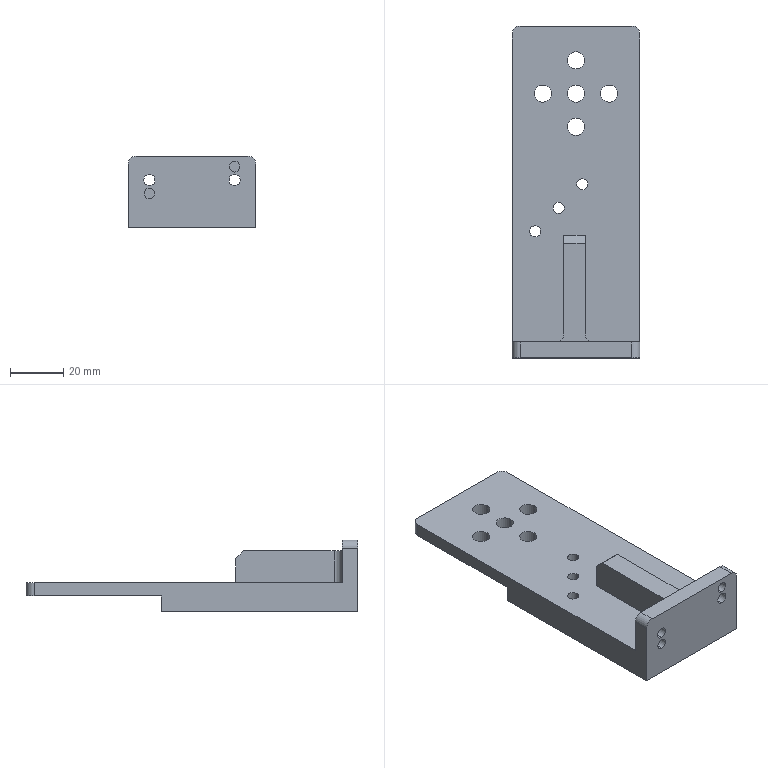NC program | NX | posted with a generic post | part box 48 x 124.7 x 27 mm
Lines 1859 to 3165 of 3165:
(ZLEVEL_PROFILE , TOOL : D6)
N3698 T12 M6
N3700 G54
N3702 G17 G0 G90 X-52.15 Y10.619 B0. C0. S9500 M3
N3704 G43 Z30. H12
N3706 Z-4.5
N3708 G94 G1 X-53.05 Y10.099 F1600.
N3710 G3 X-53.35 Y9.58 R0.6
N3712 G1 Y7.573
N3714 X-51.344
N3716 G3 X-50.824 Y7.873 R0.6
N3718 G1 X-50.304 Y8.773
N3720 G0 X-52.15 Y10.619 Z-5.
N3722 G1 X-53.05 Y10.099
N3724 G3 X-53.35 Y9.58 R0.6
N3726 G1 Y7.573
N3728 X-51.344
N3730 G3 X-50.824 Y7.873 R0.6
N3732 G1 X-50.304 Y8.773
N3734 G0 X-52.15 Y10.619 Z-5.5
N3736 G1 X-53.05 Y10.099
N3738 G3 X-53.35 Y9.58 R0.6
N3740 G1 Y7.573
N3742 X-51.344
N3744 G3 X-50.824 Y7.873 R0.6
N3746 G1 X-50.304 Y8.773
N3748 G0 X-52.15 Y10.619 Z-6.
N3750 G1 X-53.05 Y10.099
N3752 G3 X-53.35 Y9.58 R0.6
N3754 G1 Y7.573
N3756 X-51.344
N3758 G3 X-50.824 Y7.873 R0.6
N3760 G1 X-50.304 Y8.773
N3762 G0 X-52.15 Y10.619 Z-6.5
N3764 G1 X-53.05 Y10.099
N3766 G3 X-53.35 Y9.58 R0.6
N3768 G1 Y7.573
N3770 X-51.344
N3772 G3 X-50.824 Y7.873 R0.6
N3774 G1 X-50.304 Y8.773
N3776 G0 X-52.15 Y10.619 Z-7.
N3778 G1 X-53.05 Y10.099
N3780 G3 X-53.35 Y9.58 R0.6
N3782 G1 Y7.573
N3784 X-51.344
N3786 G3 X-50.824 Y7.873 R0.6
N3788 G1 X-50.304 Y8.773
N3790 G0 X-52.15 Y10.619 Z-7.5
N3792 G1 X-53.05 Y10.099
N3794 G3 X-53.35 Y9.58 R0.6
N3796 G1 Y7.573
N3798 X-51.344
N3800 G3 X-50.824 Y7.873 R0.6
N3802 G1 X-50.304 Y8.773
N3804 G0 X-52.15 Y10.619 Z-8.
N3806 G1 X-53.05 Y10.099
N3808 G3 X-53.35 Y9.58 R0.6
N3810 G1 Y7.573
N3812 X-51.344
N3814 G3 X-50.824 Y7.873 R0.6
N3816 G1 X-50.304 Y8.773
N3818 G0 X-52.15 Y10.619 Z-8.5
N3820 G1 X-53.05 Y10.099
N3822 G3 X-53.35 Y9.58 R0.6
N3824 G1 Y7.573
N3826 X-51.344
N3828 G3 X-50.824 Y7.873 R0.6
N3830 G1 X-50.304 Y8.773
N3832 G0 X-52.15 Y10.619 Z-9.
N3834 G1 X-53.05 Y10.099
N3836 G3 X-53.35 Y9.58 R0.6
N3838 G1 Y7.573
N3840 X-51.344
N3842 G3 X-50.824 Y7.873 R0.6
N3844 G1 X-50.304 Y8.773
N3846 G0 X-52.15 Y10.619 Z-9.5
N3848 G1 X-53.05 Y10.099
N3850 G3 X-53.35 Y9.58 R0.6
N3852 G1 Y7.573
N3854 X-51.344
N3856 G3 X-50.824 Y7.873 R0.6
N3858 G1 X-50.304 Y8.773
N3860 G0 X-52.15 Y10.619 Z-10.
N3862 G1 X-53.05 Y10.099
N3864 G3 X-53.35 Y9.58 R0.6
N3866 G1 Y7.573
N3868 X-51.344
N3870 G3 X-50.824 Y7.873 R0.6
N3872 G1 X-50.304 Y8.773
N3874 G0 X-52.15 Y10.619 Z-10.5
N3876 G1 X-53.05 Y10.099
N3878 G3 X-53.35 Y9.58 R0.6
N3880 G1 Y7.573
N3882 X-51.344
N3884 G3 X-50.824 Y7.873 R0.6
N3886 G1 X-50.304 Y8.773
N3888 G0 X-52.15 Y10.619 Z-11.
N3890 G1 X-53.05 Y10.099
N3892 G3 X-53.35 Y9.58 R0.6
N3894 G1 Y7.573
N3896 X-51.344
N3898 G3 X-50.824 Y7.873 R0.6
N3900 G1 X-50.304 Y8.773
N3902 G0 X-52.15 Y10.619 Z-11.5
N3904 G1 X-53.05 Y10.099
N3906 G3 X-53.35 Y9.58 R0.6
N3908 G1 Y7.573
N3910 X-51.344
N3912 G3 X-50.824 Y7.873 R0.6
N3914 G1 X-50.304 Y8.773
N3916 G0 X-52.15 Y10.619 Z-12.
N3918 G1 X-53.05 Y10.099
N3920 G3 X-53.35 Y9.58 R0.6
N3922 G1 Y7.573
N3924 X-51.344
N3926 G3 X-50.824 Y7.873 R0.6
N3928 G1 X-50.304 Y8.773
N3930 G0 X-52.15 Y10.619 Z-12.5
N3932 G1 X-53.05 Y10.099
N3934 G3 X-53.35 Y9.58 R0.6
N3936 G1 Y7.573
N3938 X-51.344
N3940 G3 X-50.824 Y7.873 R0.6
N3942 G1 X-50.304 Y8.773
N3944 G0 X-52.15 Y10.619 Z-13.
N3946 G1 X-53.05 Y10.099
N3948 G3 X-53.35 Y9.58 R0.6
N3950 G1 Y7.573
N3952 X-51.344
N3954 G3 X-50.824 Y7.873 R0.6
N3956 G1 X-50.304 Y8.773
N3958 G0 X-52.15 Y10.619 Z-13.5
N3960 G1 X-53.05 Y10.099
N3962 G3 X-53.35 Y9.58 R0.6
N3964 G1 Y7.573
N3966 X-51.344
N3968 G3 X-50.824 Y7.873 R0.6
N3970 G1 X-50.304 Y8.773
N3972 G0 X-52.15 Y10.619 Z-14.
N3974 G1 X-53.05 Y10.099
N3976 G3 X-53.35 Y9.58 R0.6
N3978 G1 Y7.573
N3980 X-51.344
N3982 G3 X-50.824 Y7.873 R0.6
N3984 G1 X-50.304 Y8.773
N3986 G0 X-52.15 Y10.619 Z-14.5
N3988 G1 X-53.05 Y10.099
N3990 G3 X-53.35 Y9.58 R0.6
N3992 G1 Y7.573
N3994 X-51.344
N3996 G3 X-50.824 Y7.873 R0.6
N3998 G1 X-50.304 Y8.773
N4000 G0 X-52.15 Y10.619 Z-15.
N4002 G1 X-53.05 Y10.099
N4004 G3 X-53.35 Y9.58 R0.6
N4006 G1 Y7.573
N4008 X-51.344
N4010 G3 X-50.824 Y7.873 R0.6
N4012 G1 X-50.304 Y8.773
N4014 G0 X-52.15 Y10.619 Z-15.5
N4016 G1 X-53.05 Y10.099
N4018 G3 X-53.35 Y9.58 R0.6
N4020 G1 Y7.573
N4022 X-51.344
N4024 G3 X-50.824 Y7.873 R0.6
N4026 G1 X-50.304 Y8.773
N4028 G0 X-52.15 Y10.619 Z-16.
N4030 G1 X-53.05 Y10.099
N4032 G3 X-53.35 Y9.58 R0.6
N4034 G1 Y7.573
N4036 X-51.344
N4038 G3 X-50.824 Y7.873 R0.6
N4040 G1 X-50.304 Y8.773
N4042 G0 Z30.
N4044 Y-7.627
N4046 Z-4.5
N4048 G1 X-50.824 Y-6.727
N4050 G3 X-51.344 Y-6.427 R0.6
N4052 G1 X-53.35
N4054 Y-8.433
N4056 G3 X-53.05 Y-8.953 R0.6
N4058 G1 X-52.15 Y-9.472
N4060 G0 X-50.304 Y-7.627 Z-5.
N4062 G1 X-50.824 Y-6.727
N4064 G3 X-51.344 Y-6.427 R0.6
N4066 G1 X-53.35
N4068 Y-8.433
N4070 G3 X-53.05 Y-8.953 R0.6
N4072 G1 X-52.15 Y-9.472
N4074 G0 X-50.304 Y-7.627 Z-5.5
N4076 G1 X-50.824 Y-6.727
N4078 G3 X-51.344 Y-6.427 R0.6
N4080 G1 X-53.35
N4082 Y-8.433
N4084 G3 X-53.05 Y-8.953 R0.6
N4086 G1 X-52.15 Y-9.472
N4088 G0 X-50.304 Y-7.627 Z-6.
N4090 G1 X-50.824 Y-6.727
N4092 G3 X-51.344 Y-6.427 R0.6
N4094 G1 X-53.35
N4096 Y-8.433
N4098 G3 X-53.05 Y-8.953 R0.6
N4100 G1 X-52.15 Y-9.472
N4102 G0 X-50.304 Y-7.627 Z-6.5
N4104 G1 X-50.824 Y-6.727
N4106 G3 X-51.344 Y-6.427 R0.6
N4108 G1 X-53.35
N4110 Y-8.433
N4112 G3 X-53.05 Y-8.953 R0.6
N4114 G1 X-52.15 Y-9.472
N4116 G0 X-50.304 Y-7.627 Z-7.
N4118 G1 X-50.824 Y-6.727
N4120 G3 X-51.344 Y-6.427 R0.6
N4122 G1 X-53.35
N4124 Y-8.433
N4126 G3 X-53.05 Y-8.953 R0.6
N4128 G1 X-52.15 Y-9.472
N4130 G0 X-50.304 Y-7.627 Z-7.5
N4132 G1 X-50.824 Y-6.727
N4134 G3 X-51.344 Y-6.427 R0.6
N4136 G1 X-53.35
N4138 Y-8.433
N4140 G3 X-53.05 Y-8.953 R0.6
N4142 G1 X-52.15 Y-9.472
N4144 G0 X-50.304 Y-7.627 Z-8.
N4146 G1 X-50.824 Y-6.727
N4148 G3 X-51.344 Y-6.427 R0.6
N4150 G1 X-53.35
N4152 Y-8.433
N4154 G3 X-53.05 Y-8.953 R0.6
N4156 G1 X-52.15 Y-9.472
N4158 G0 X-50.304 Y-7.627 Z-8.5
N4160 G1 X-50.824 Y-6.727
N4162 G3 X-51.344 Y-6.427 R0.6
N4164 G1 X-53.35
N4166 Y-8.433
N4168 G3 X-53.05 Y-8.953 R0.6
N4170 G1 X-52.15 Y-9.472
N4172 G0 X-50.304 Y-7.627 Z-9.
N4174 G1 X-50.824 Y-6.727
N4176 G3 X-51.344 Y-6.427 R0.6
N4178 G1 X-53.35
N4180 Y-8.433
N4182 G3 X-53.05 Y-8.953 R0.6
N4184 G1 X-52.15 Y-9.472
N4186 G0 X-50.304 Y-7.627 Z-9.5
N4188 G1 X-50.824 Y-6.727
N4190 G3 X-51.344 Y-6.427 R0.6
N4192 G1 X-53.35
N4194 Y-8.433
N4196 G3 X-53.05 Y-8.953 R0.6
N4198 G1 X-52.15 Y-9.472
N4200 G0 X-50.304 Y-7.627 Z-10.
N4202 G1 X-50.824 Y-6.727
N4204 G3 X-51.344 Y-6.427 R0.6
N4206 G1 X-53.35
N4208 Y-8.433
N4210 G3 X-53.05 Y-8.953 R0.6
N4212 G1 X-52.15 Y-9.472
N4214 G0 X-50.304 Y-7.627 Z-10.5
N4216 G1 X-50.824 Y-6.727
N4218 G3 X-51.344 Y-6.427 R0.6
N4220 G1 X-53.35
N4222 Y-8.433
N4224 G3 X-53.05 Y-8.953 R0.6
N4226 G1 X-52.15 Y-9.472
N4228 G0 X-50.304 Y-7.627 Z-11.
N4230 G1 X-50.824 Y-6.727
N4232 G3 X-51.344 Y-6.427 R0.6
N4234 G1 X-53.35
N4236 Y-8.433
N4238 G3 X-53.05 Y-8.953 R0.6
N4240 G1 X-52.15 Y-9.472
N4242 G0 X-50.304 Y-7.627 Z-11.5
N4244 G1 X-50.824 Y-6.727
N4246 G3 X-51.344 Y-6.427 R0.6
N4248 G1 X-53.35
N4250 Y-8.433
N4252 G3 X-53.05 Y-8.953 R0.6
N4254 G1 X-52.15 Y-9.472
N4256 G0 X-50.304 Y-7.627 Z-12.
N4258 G1 X-50.824 Y-6.727
N4260 G3 X-51.344 Y-6.427 R0.6
N4262 G1 X-53.35
N4264 Y-8.433
N4266 G3 X-53.05 Y-8.953 R0.6
N4268 G1 X-52.15 Y-9.472
N4270 G0 X-50.304 Y-7.627 Z-12.5
N4272 G1 X-50.824 Y-6.727
N4274 G3 X-51.344 Y-6.427 R0.6
N4276 G1 X-53.35
N4278 Y-8.433
N4280 G3 X-53.05 Y-8.953 R0.6
N4282 G1 X-52.15 Y-9.472
N4284 G0 X-50.304 Y-7.627 Z-13.
N4286 G1 X-50.824 Y-6.727
N4288 G3 X-51.344 Y-6.427 R0.6
N4290 G1 X-53.35
N4292 Y-8.433
N4294 G3 X-53.05 Y-8.953 R0.6
N4296 G1 X-52.15 Y-9.472
N4298 G0 X-50.304 Y-7.627 Z-13.5
N4300 G1 X-50.824 Y-6.727
N4302 G3 X-51.344 Y-6.427 R0.6
N4304 G1 X-53.35
N4306 Y-8.433
N4308 G3 X-53.05 Y-8.953 R0.6
N4310 G1 X-52.15 Y-9.472
N4312 G0 X-50.304 Y-7.627 Z-14.
N4314 G1 X-50.824 Y-6.727
N4316 G3 X-51.344 Y-6.427 R0.6
N4318 G1 X-53.35
N4320 Y-8.433
N4322 G3 X-53.05 Y-8.953 R0.6
N4324 G1 X-52.15 Y-9.472
N4326 G0 X-50.304 Y-7.627 Z-14.5
N4328 G1 X-50.824 Y-6.727
N4330 G3 X-51.344 Y-6.427 R0.6
N4332 G1 X-53.35
N4334 Y-8.433
N4336 G3 X-53.05 Y-8.953 R0.6
N4338 G1 X-52.15 Y-9.472
N4340 G0 X-50.304 Y-7.627 Z-15.
N4342 G1 X-50.824 Y-6.727
N4344 G3 X-51.344 Y-6.427 R0.6
N4346 G1 X-53.35
N4348 Y-8.433
N4350 G3 X-53.05 Y-8.953 R0.6
N4352 G1 X-52.15 Y-9.472
N4354 G0 X-50.304 Y-7.627 Z-15.5
N4356 G1 X-50.824 Y-6.727
N4358 G3 X-51.344 Y-6.427 R0.6
N4360 G1 X-53.35
N4362 Y-8.433
N4364 G3 X-53.05 Y-8.953 R0.6
N4366 G1 X-52.15 Y-9.472
N4368 G0 X-50.304 Y-7.627 Z-16.
N4370 G1 X-50.824 Y-6.727
N4372 G3 X-51.344 Y-6.427 R0.6
N4374 G1 X-53.35
N4376 Y-8.433
N4378 G3 X-53.05 Y-8.953 R0.6
N4380 G1 X-52.15 Y-9.472
N4382 G0 Z30.
N4384 M5
(ZLEVEL_PROFILE_1 , TOOL : D6R0.5)
N4386 T16 M6
N4388 G54
N4390 G17 G0 G90 X-65.841 Y25.724 B0. C0. S9500 M3
N4392 G43 Z30. H16
N4394 Z2.992
N4396 G94 G1 Z-0.008 F3500.
N4398 G3 X-62.85 Y23.619 R3.
N4400 G1 X-62.35 Y23.73
N4402 X-56.35
N4404 X-55.858 Y23.68
N4406 X-55.852 Y23.65
N4408 X-55.847 Y23.757 Z-0.017
N4410 X-55.857 Y23.784
N4412 X-56.35 Y23.843
N4414 X-62.35
N4416 X-62.85 Y23.754
N4418 Y23.841 Z-0.023
N4420 Y23.884 Z-0.029
N4422 X-62.35 Y23.947
N4424 X-56.35
N4426 X-55.848 Y23.894
N4428 X-55.851 Y23.951 Z-0.036
N4430 X-55.852 Y23.992 Z-0.043
N4432 X-56.35 Y24.049
N4434 X-62.35
N4436 X-62.85 Y23.971
N4438 X-62.849 Y24.049 Z-0.052
N4440 Y24.074 Z-0.061
N4442 X-62.35 Y24.149
N4444 X-56.35
N4446 X-55.796 Y24.088
N4448 X-55.711 Y24.068
N4450 X-55.78 Y24.135 Z-0.071
N4452 X-55.85 Y24.197 Z-0.08
N4454 X-56.35 Y24.246
N4456 X-62.35
N4458 X-62.812 Y24.203
N4460 X-62.85 Y24.194
N4462 X-62.865 Y24.245 Z-0.092
N4464 X-62.876 Y24.281 Z-0.103
N4466 X-62.35 Y24.344
N4468 X-56.35
N4470 X-55.79 Y24.271
N4472 X-55.719 Y24.359 Z-0.129
N4474 X-56.35 Y24.441
N4476 X-62.35
N4478 X-62.907 Y24.377
N4480 X-62.932 Y24.424 Z-0.143
N4482 X-62.917 Y24.429
N4484 X-62.35 Y24.492
N4486 X-56.35
N4488 X-55.691 Y24.406
N4490 X-55.678 Y24.447 Z-0.157
N4492 X-55.667 Y24.483 Z-0.17
N4494 X-56.35 Y24.577
N4496 X-62.35
N4498 X-62.917 Y24.514
N4500 X-62.993 Y24.491
N4502 X-62.946 Y24.603 Z-0.202
N4504 X-62.917 Y24.611
N4506 X-62.35 Y24.672
N4508 X-56.35
N4510 X-55.706 Y24.59
N4512 X-55.753 Y24.684 Z-0.237
N4514 X-56.35 Y24.766
N4516 X-62.35
N4518 X-62.897 Y24.701
N4520 X-62.872 Y24.797 Z-0.274
N4522 X-62.35 Y24.858
N4524 X-56.35
N4526 X-55.804 Y24.788
N4528 X-55.85 Y24.9 Z-0.314
N4530 X-56.35 Y24.949
N4532 X-62.35
N4534 X-62.856 Y24.901
N4536 X-62.917 Y24.964 Z-0.35
N4538 X-62.871 Y24.972
N4540 X-62.35 Y25.025
N4542 X-56.35
N4544 X-55.851 Y24.965
N4546 Y25.021 Z-0.371
N4548 Y25.048 Z-0.393
N4550 X-56.35 Y25.111
N4552 X-62.35
N4554 X-62.826 Y25.069
N4556 X-62.917 Y25.051
N4558 X-62.869 Y25.148 Z-0.44
N4560 X-62.35 Y25.199
N4562 X-56.35
N4564 X-55.851 Y25.139
N4566 X-55.85 Y25.197 Z-0.465
N4568 Y25.239 Z-0.489
N4570 X-56.35 Y25.285
N4572 X-62.35
N4574 X-62.85 Y25.239
N4576 Y25.283 Z-0.515
N4578 Y25.313 Z-0.541
N4580 X-62.35 Y25.37
N4582 X-56.35
N4584 X-55.851 Y25.312
N4586 Y25.366 Z-0.569
N4588 Y25.393 Z-0.596
N4590 X-56.35 Y25.454
N4592 X-62.35
N4594 X-62.849 Y25.394
N4596 Y25.449 Z-0.624
N4598 Y25.478 Z-0.653
N4600 X-62.35 Y25.536
N4602 X-56.35
N4604 X-55.851 Y25.477
N4606 Y25.53 Z-0.682
N4608 Y25.566 Z-0.712
N4610 X-55.943 Y25.584
N4612 X-56.35 Y25.616
N4614 X-62.35
N4616 X-62.849 Y25.566
N4618 X-62.85 Y25.61 Z-0.743
N4620 Y25.644 Z-0.773
N4622 X-62.35 Y25.694
N4624 X-56.35
N4626 X-55.85 Y25.642
N4628 Y25.688 Z-0.805
N4630 X-55.849 Y25.719 Z-0.837
N4632 G3 X-56.35 Y25.771 R2.789
N4634 G1 X-62.35
N4636 G3 X-62.851 Y25.721 R3.458
N4638 G1 Y25.764 Z-0.87
N4640 X-62.85 Y25.796 Z-0.903
N4642 X-62.35 Y25.846
N4644 X-56.35
N4646 G2 X-55.85 Y25.794 R2.997
N4648 G1 Y25.838 Z-0.937
N4650 Y25.871 Z-0.971
N4652 G3 X-56.35 Y25.919 R3.27
N4654 G1 X-62.35
N4656 G3 X-62.85 Y25.869 R3.49
N4658 G1 Y25.91 Z-1.006
N4660 Y25.942 Z-1.041
N4662 G2 X-62.35 Y25.99 R3.793
N4664 G1 X-56.35
N4666 X-55.85 Y25.948
N4668 X-55.849 Y25.98 Z-1.077
N4670 Y26.013 Z-1.113
N4672 X-56.35 Y26.06
N4674 X-62.35
N4676 G3 X-62.85 Y26.009 R3.602
N4678 G1 X-62.851 Y26.049 Z-1.15
N4680 Y26.078 Z-1.187
N4682 G2 X-62.35 Y26.127 R3.586
N4684 G1 X-56.35
N4686 G2 X-55.849 Y26.079 R3.257
N4688 G1 Y26.115 Z-1.225
N4690 Y26.144 Z-1.263
N4692 G3 X-56.35 Y26.192 R3.472
N4694 G1 X-62.35
N4696 G3 X-62.851 Y26.143 R3.822
N4698 G1 X-62.85 Y26.179 Z-1.302
N4700 Y26.206 Z-1.341
N4702 G2 X-62.35 Y26.254 R3.729
N4704 G1 X-56.35
N4706 G2 X-55.849 Y26.209 R4.005
N4708 G1 Y26.242 Z-1.38
N4710 X-55.85 Y26.273 Z-1.42
N4712 G3 X-56.35 Y26.315 R5.086
N4714 G1 X-62.35
N4716 G3 X-62.85 Y26.271 R3.593
N4718 G1 Y26.301 Z-1.461
N4720 Y26.325 Z-1.501
N4722 G2 X-62.35 Y26.373 R3.994
N4724 G1 X-56.35
N4726 X-55.849 Y26.331
N4728 Y26.357 Z-1.543
N4730 X-55.848 Y26.385 Z-1.584
N4732 G3 X-56.35 Y26.429 R4.
N4734 G1 X-62.35
N4736 G3 X-62.851 Y26.38 R3.678
N4738 G1 Y26.412 Z-1.626
N4740 X-62.852 Y26.434 Z-1.668
N4742 G2 X-62.35 Y26.483 R3.802
N4744 G1 X-56.35
N4746 G2 X-55.848 Y26.439 R3.93
N4748 G1 Y26.464 Z-1.711
N4750 Y26.491 Z-1.754
N4752 X-56.35 Y26.534
N4754 X-62.35
N4756 G3 X-62.851 Y26.485 R3.963
N4758 G1 Y26.514 Z-1.798
N4760 Y26.533 Z-1.842
N4762 G2 X-62.35 Y26.582 R3.824
N4764 G1 X-56.35
N4766 X-55.848 Y26.542
N4768 Y26.562 Z-1.886
N4770 X-55.849 Y26.59 Z-1.93
N4772 G3 X-56.35 Y26.628 R5.022
N4774 G1 X-62.35
N4776 G3 X-62.85 Y26.582 R3.689
N4778 G1 Y26.608 Z-1.975
N4780 Y26.629 Z-2.02
N4782 G2 X-62.35 Y26.672 R4.731
N4784 G1 X-56.35
N4786 G2 X-55.849 Y26.633 R4.583
N4788 G1 Y26.649 Z-2.066
N4790 X-55.848 Y26.673 Z-2.112
N4792 G3 X-56.35 Y26.713 R4.549
N4794 G1 X-62.35
N4796 X-62.851 Y26.666
N4798 X-62.852 Y26.688 Z-2.158
N4800 Y26.704 Z-2.204
N4802 G2 X-62.35 Y26.751 R4.392
N4804 G1 X-56.35
N4806 G2 X-55.847 Y26.711 R4.65
N4808 G1 X-55.846 Y26.725 Z-2.251
N4810 Y26.748 Z-2.297
N4812 G3 X-56.35 Y26.787 R4.816
N4814 G1 X-62.35
N4816 G3 X-62.854 Y26.742 R4.237
N4818 G1 Y26.76 Z-2.344
N4820 Y26.78 Z-2.392
N4822 G2 X-62.35 Y26.82 R4.793
N4824 G1 X-56.35
N4826 X-55.846 Y26.784
N4828 Y26.794 Z-2.439
N4830 Y26.815 Z-2.487
N4832 X-56.35 Y26.85
N4834 X-62.35
N4836 G3 X-62.854 Y26.811 R5.221
N4838 G1 Y26.82 Z-2.535
N4840 X-62.855 Y26.837 Z-2.583
N4842 G2 X-62.35 Y26.878 R4.638
N4844 G1 X-56.35
N4846 X-55.846 Y26.843
N4848 Y26.848 Z-2.632
N4850 Y26.87 Z-2.68
N4852 X-56.35 Y26.903
N4854 X-62.35
N4856 G3 X-62.854 Y26.862 R4.647
N4858 G1 Y26.871 Z-2.729
N4860 Y26.887 Z-2.778
N4862 G2 X-62.35 Y26.925 R5.028
N4864 G1 X-56.35
N4866 X-55.848 Y26.895
N4868 Y26.901 Z-2.827
N4870 X-55.849 Y26.919 Z-2.876
N4872 X-56.35 Y26.944
N4874 X-62.35
N4876 X-62.852 Y26.911
N4878 Y26.917 Z-2.925
N4880 X-62.851 Y26.933 Z-2.974
N4882 X-62.35 Y26.96
N4884 X-56.35
N4886 X-55.85 Y26.937
N4888 Y26.947 Z-3.024
N4890 Y26.953 Z-3.073
N4892 X-56.35 Y26.974
N4894 X-62.35
N4896 X-62.85 Y26.95
N4898 Y26.958 Z-3.123
N4900 Y26.967 Z-3.173
N4902 X-62.35 Y26.985
N4904 X-56.35
N4906 X-55.868 Y26.968
N4908 Y26.976 Z-3.255
N4910 X-56.35 Y26.991
N4912 X-62.35
N4914 X-62.85 Y26.976
N4916 Y26.985 Z-3.336
N4918 X-62.35 Y26.996
N4920 X-56.35
N4922 X-55.868 Y26.984
N4924 Y26.992 Z-3.418
N4926 X-56.384 Y26.998
N4928 X-62.573 Y26.997
N4930 X-62.85 Y26.994
N4932 Y26.997 Z-3.5
N4934 X-62.229 Y26.998
N4936 X-56.384
N4938 X-55.868 Y26.996
N4940 G3 X-52.95 Y29.254 R3.
N4942 G1 Z-0.5
N4944 G0 Z30.
N4946 X-52.68 Y-25.576
N4948 Z2.992
N4950 G1 Z-0.008
N4952 G3 X-55.848 Y-23.659 R3.
N4954 G1 X-55.867 Y-23.682
N4956 X-56.35 Y-23.73
N4958 X-62.35
N4960 X-62.85 Y-23.619
N4962 Y-23.739 Z-0.012
N4964 Y-23.754 Z-0.017
N4966 X-62.35 Y-23.843
N4968 X-56.35
N4970 X-55.848 Y-23.775
N4972 X-55.85 Y-23.849 Z-0.023
N4974 X-55.851 Y-23.883 Z-0.029
N4976 X-56.35 Y-23.947
N4978 X-62.35
N4980 X-62.85 Y-23.891
N4982 X-62.855 Y-23.95 Z-0.036
N4984 X-62.858 Y-23.991 Z-0.043
N4986 X-62.35 Y-24.049
N4988 X-56.35
N4990 X-55.851 Y-23.97
N4992 Y-24.049 Z-0.052
N4994 Y-24.073 Z-0.061
N4996 X-56.35 Y-24.149
N4998 X-62.35
N5000 X-62.874 Y-24.094
N5002 X-63.001 Y-24.066
N5004 X-62.928 Y-24.134 Z-0.071
N5006 X-62.855 Y-24.196 Z-0.08
N5008 X-62.846 Y-24.198
N5010 X-62.35 Y-24.246
N5012 X-56.35
N5014 X-55.851 Y-24.194
N5016 X-55.794 Y-24.271 Z-0.103
N5018 X-56.35 Y-24.344
N5020 X-62.35
N5022 X-62.876 Y-24.281
N5024 X-62.893 Y-24.334 Z-0.116
N5026 X-62.907 Y-24.377 Z-0.129
N5028 X-62.35 Y-24.441
N5030 X-56.35
N5032 X-55.727 Y-24.359
N5034 X-55.694 Y-24.408 Z-0.143
N5036 X-56.35 Y-24.492
N5038 X-62.35
N5040 G2 X-63.089 Y-24.373 R2.416
N5042 G1 Y-24.46 Z-0.17
N5044 G3 X-62.35 Y-24.577 R2.465
N5046 G1 X-56.35
N5048 X-55.674 Y-24.486
N5050 X-55.707 Y-24.59 Z-0.202
N5052 X-56.35 Y-24.672
N5054 X-62.35
N5056 X-62.917 Y-24.611
N5058 X-62.95 Y-24.602
N5060 X-62.85 Y-24.673 Z-0.22
N5062 X-62.745 Y-24.721 Z-0.237
N5064 X-62.35 Y-24.766
N5066 X-56.35
N5068 X-55.754 Y-24.684
N5070 X-55.804 Y-24.788 Z-0.274
N5072 X-56.35 Y-24.858
N5074 X-62.35
N5076 X-62.745 Y-24.817
N5078 X-62.848 Y-24.903 Z-0.314
N5080 X-62.799 Y-24.911
N5082 X-62.35 Y-24.949
N5084 X-56.35
N5086 X-55.85 Y-24.9
N5088 X-55.851 Y-24.94 Z-0.332
N5090 Y-24.965 Z-0.35
N5092 X-56.35 Y-25.025
N5094 X-62.35
N5096 X-62.865 Y-24.974
N5098 X-62.917 Y-24.964
N5100 Y-25.008 Z-0.371
N5102 Y-25.051 Z-0.393
N5104 X-62.82 Y-25.07
N5106 X-62.35 Y-25.111
N5108 X-56.35
N5110 X-55.851 Y-25.048
N5112 Y-25.109 Z-0.416
N5114 Y-25.139 Z-0.44
N5116 X-56.35 Y-25.199
N5118 X-62.35
N5120 X-62.832 Y-25.156
N5122 X-62.864 Y-25.149
N5124 X-62.789 Y-25.207 Z-0.465
N5126 X-62.712 Y-25.255 Z-0.489
N5128 X-62.35 Y-25.285
N5130 X-56.35
N5132 X-55.85 Y-25.239
N5134 Y-25.283 Z-0.515
N5136 X-55.851 Y-25.312 Z-0.541
N5138 X-56.35 Y-25.37
N5140 X-62.35
N5142 X-62.745 Y-25.328
N5144 Y-25.383 Z-0.569
N5146 Y-25.409 Z-0.596
N5148 X-62.35 Y-25.454
N5150 X-56.35
N5152 X-55.851 Y-25.393
N5154 Y-25.449 Z-0.624
N5156 Y-25.477 Z-0.653
N5158 X-56.35 Y-25.536
N5160 X-62.35
N5162 X-62.745 Y-25.494
N5164 X-62.831 Y-25.569 Z-0.712
N5166 X-62.35 Y-25.616
N5168 X-56.35
N5170 X-55.943 Y-25.584
N5172 X-55.851 Y-25.566
N5174 X-55.85 Y-25.611 Z-0.743
N5176 Y-25.642 Z-0.773
N5178 X-56.35 Y-25.694
N5180 X-62.35
N5182 X-62.85 Y-25.644
N5184 Y-25.688 Z-0.805
N5186 X-62.851 Y-25.721 Z-0.837
N5188 G3 X-62.35 Y-25.771 R3.653
N5190 G1 X-56.35
N5192 G3 X-55.849 Y-25.719 R3.635
N5194 G1 Y-25.764 Z-0.87
N5196 X-55.85 Y-25.794 Z-0.903
N5198 G2 X-56.35 Y-25.846 R2.997
N5200 G1 X-62.35
N5202 X-62.85 Y-25.796
N5204 Y-25.839 Z-0.937
N5206 Y-25.869 Z-0.971
N5208 G3 X-62.35 Y-25.919 R4.135
N5210 G1 X-56.35
N5212 G3 X-55.85 Y-25.871 R5.06
N5214 G1 Y-25.91 Z-1.006
N5216 Y-25.948 Z-1.041
N5218 X-56.35 Y-25.99
N5220 X-62.35
N5222 G2 X-62.85 Y-25.942 R4.519
N5224 G1 Y-25.982 Z-1.077
N5226 Y-26.009 Z-1.113
N5228 G3 X-62.35 Y-26.06 R3.602
N5230 G1 X-56.35
N5232 X-55.849 Y-26.013
N5234 Y-26.049 Z-1.15
N5236 Y-26.079 Z-1.187
N5238 G2 X-56.35 Y-26.127 R4.069
N5240 G1 X-62.35
N5242 G2 X-62.851 Y-26.078 R4.524
N5244 G1 Y-26.115 Z-1.225
N5246 Y-26.143 Z-1.263
N5248 G3 X-62.35 Y-26.192 R4.457
N5250 G1 X-56.35
N5252 G3 X-55.849 Y-26.144 R4.038
N5254 G1 Y-26.179 Z-1.302
N5256 Y-26.209 Z-1.341
N5258 G2 X-56.35 Y-26.254 R3.723
N5260 G1 X-62.35
N5262 G2 X-62.85 Y-26.206 R4.725
N5264 G1 Y-26.242 Z-1.38
N5266 Y-26.271 Z-1.42
N5268 G3 X-62.35 Y-26.315 R3.593
N5270 G1 X-56.35
N5272 G3 X-55.85 Y-26.273 R18.177
N5274 G1 X-55.849 Y-26.301 Z-1.461
N5276 Y-26.331 Z-1.501
N5278 X-56.35 Y-26.373
N5280 X-62.35
N5282 G2 X-62.85 Y-26.325 R3.994
N5284 G1 X-62.851 Y-26.357 Z-1.543
N5286 Y-26.38 Z-1.584
N5288 G3 X-62.35 Y-26.429 R3.678
N5290 G1 X-56.35
N5292 G3 X-55.848 Y-26.385 R4.564
N5294 G1 Y-26.412 Z-1.626
N5296 Y-26.439 Z-1.668
N5298 G2 X-56.35 Y-26.483 R7.17
N5300 G1 X-62.35
N5302 G2 X-62.852 Y-26.434 R3.802
N5304 G1 X-62.851 Y-26.464 Z-1.711
N5306 Y-26.485 Z-1.754
N5308 G3 X-62.35 Y-26.534 R3.965
N5310 G1 X-56.35
N5312 X-55.848 Y-26.491
N5314 Y-26.514 Z-1.798
N5316 Y-26.542 Z-1.842
N5318 X-56.35 Y-26.582
N5320 X-62.35
N5322 G2 X-62.851 Y-26.533 R3.829
N5324 G1 Y-26.562 Z-1.886
N5326 X-62.85 Y-26.582 Z-1.93
N5328 G3 X-62.35 Y-26.628 R3.697
N5330 G1 X-56.35
N5332 G3 X-55.849 Y-26.59 R5.024
N5334 G1 Y-26.607 Z-1.975
N5336 Y-26.633 Z-2.02
N5338 G2 X-56.35 Y-26.672 R4.579
N5340 G1 X-62.35
N5342 G2 X-62.85 Y-26.629 R5.538
N5344 G1 X-62.851 Y-26.65 Z-2.066
N5346 Y-26.666 Z-2.112
N5348 X-62.35 Y-26.713
N5350 X-56.35
N5352 G3 X-55.848 Y-26.673 R4.594
N5354 G1 X-55.847 Y-26.688 Z-2.158
N5356 Y-26.71 Z-2.204
N5358 G2 X-56.35 Y-26.751 R4.641
N5360 G1 X-62.35
N5362 G2 X-62.852 Y-26.704 R6.058
N5364 G1 X-62.853 Y-26.725 Z-2.251
N5366 X-62.854 Y-26.743 Z-2.297
N5368 G3 X-62.35 Y-26.787 R4.297
N5370 G1 X-56.35
N5372 G3 X-55.846 Y-26.747 R4.803
N5374 G1 Y-26.76 Z-2.344
N5376 X-55.845 Y-26.783 Z-2.392
N5378 X-56.35 Y-26.82
N5380 X-62.35
N5382 G2 X-62.854 Y-26.78 R5.376
N5384 G1 Y-26.794 Z-2.439
N5386 Y-26.813 Z-2.487
N5388 G3 X-62.35 Y-26.85 R5.58
N5390 G1 X-56.35
N5392 X-55.846 Y-26.815
N5394 Y-26.82 Z-2.535
N5396 Y-26.841 Z-2.583
N5398 X-56.35 Y-26.878
N5400 X-62.35
N5402 G2 X-62.854 Y-26.84 R6.091
N5404 G1 Y-26.848 Z-2.632
N5406 Y-26.867 Z-2.68
N5408 G3 X-62.35 Y-26.903 R6.146
N5410 G1 X-56.35
N5412 X-55.846 Y-26.866
N5414 Y-26.871 Z-2.729
N5416 X-55.847 Y-26.889 Z-2.778
N5418 X-56.35 Y-26.925
N5420 X-62.35
N5422 X-62.853 Y-26.894
N5424 X-62.852 Y-26.901 Z-2.827
N5426 X-62.851 Y-26.919 Z-2.876
N5428 X-62.35 Y-26.944
N5430 X-56.35
N5432 X-55.848 Y-26.909
N5434 Y-26.917 Z-2.925
N5436 X-55.849 Y-26.928 Z-2.974
N5438 X-56.35 Y-26.96
N5440 X-62.35
N5442 X-62.851 Y-26.938
N5444 X-62.85 Y-26.947 Z-3.024
N5446 Y-26.955 Z-3.073
N5448 X-62.35 Y-26.974
N5450 X-56.35
N5452 X-55.849 Y-26.948
N5454 X-55.936 Y-26.969 Z-3.173
N5456 X-56.35 Y-26.985
N5458 X-62.35
N5460 X-62.85 Y-26.97
N5462 Y-26.978 Z-3.255
N5464 X-62.35 Y-26.991
N5466 X-56.35
N5468 X-55.868 Y-26.975
N5470 Y-26.983 Z-3.336
N5472 X-56.35 Y-26.996
N5474 X-62.35
N5476 X-62.85 Y-26.986
N5478 Y-26.994 Z-3.418
N5480 X-62.35 Y-26.999
N5482 X-56.35
N5484 X-55.868 Y-26.992
N5486 Y-26.997 Z-3.5
N5488 X-56.384 Y-27.
N5490 X-62.85 Y-26.999
N5492 G3 X-65.755 Y-29.251 R3.
N5494 G1 Z-0.5
N5496 G0 Z30.
(ZLEVEL_PROFILE_1_COPY , TOOL : D6R0.5)
N5498 X-14.362 Y7.986
N5500 Z-1.071
N5502 G1 Z-4.071
N5504 G3 X-16.575 Y5.045 R3.
N5506 G1 X-16.572 Y4.875
N5508 Y-3.728
N5510 X-16.575 Y-3.899
N5512 X-16.537 Z-4.106
N5514 X-16.504 Y-3.9 Z-4.141
N5516 X-16.501 Y-3.728
N5518 Y4.875
N5520 X-16.504 Y5.046
N5522 X-16.466 Z-4.177
N5524 X-16.433 Z-4.212
N5526 X-16.431 Y4.573
N5528 Y-3.427
N5530 X-16.433 Y-3.9
N5532 X-16.395 Z-4.247
N5534 X-16.363 Z-4.283
N5536 X-16.36 Y-3.427
N5538 Y4.573
N5540 X-16.363 Y5.047
N5542 X-16.325 Z-4.318
N5544 X-16.292 Z-4.354
N5546 X-16.289 Y4.573
N5548 Y-3.427
N5550 X-16.292 Y-3.901
N5552 X-16.254 Z-4.389
N5554 X-16.221 Z-4.424
N5556 X-16.219 Y-3.427
N5558 Y4.573
N5560 X-16.221 Y5.047
N5562 X-16.183 Y5.048 Z-4.46
N5564 X-16.15 Z-4.495
N5566 X-16.148 Y4.573
N5568 Y-3.427
N5570 X-16.15 Y-3.901
N5572 X-16.113 Y-3.902 Z-4.53
N5574 X-16.08 Z-4.566
N5576 X-16.077 Y-3.427
N5578 Y4.573
N5580 X-16.08 Y5.048
N5582 X-16.042 Z-4.601
N5584 X-16.009 Y5.049 Z-4.636
N5586 X-16.006 Y4.573
N5588 Y-3.427
N5590 X-16.009 Y-3.902
N5592 X-15.971 Z-4.672
N5594 X-15.938 Y-3.903 Z-4.707
N5596 X-15.936 Y-3.427
N5598 Y4.573
N5600 X-15.938 Y5.049
N5602 X-15.9 Z-4.742
N5604 X-15.868 Z-4.778
N5606 X-15.865 Y4.573
N5608 Y-3.427
N5610 X-15.868 Y-3.903
N5612 X-15.83 Z-4.813
N5614 X-15.797 Z-4.849
N5616 X-15.794 Y-3.427
N5618 Y4.573
N5620 X-15.797 Y5.05
N5622 X-15.759 Z-4.884
N5624 X-15.726 Z-4.919
N5626 X-15.724 Y4.573
N5628 Y-3.427
N5630 X-15.726 Y-3.904
N5632 X-15.688 Z-4.955
N5634 X-15.655 Z-4.99
N5636 X-15.653 Y-3.427
N5638 Y4.573
N5640 X-15.655 Y5.051
N5642 X-15.618 Z-5.025
N5644 X-15.585 Z-5.061
N5646 X-15.582 Y4.573
N5648 Y-3.427
N5650 X-15.585 Y-3.904
N5652 X-15.547 Y-3.905 Z-5.096
N5654 X-15.514 Z-5.131
N5656 X-15.512 Y-3.427
N5658 Y4.573
N5660 X-15.514 Y5.051
N5662 X-15.476 Z-5.167
N5664 X-15.443 Z-5.202
N5666 X-15.441 Y4.573
N5668 Y-3.427
N5670 X-15.443 Y-3.905
N5672 X-15.405 Z-5.237
N5674 X-15.373 Z-5.273
N5676 X-15.37 Y-3.427
N5678 Y4.573
N5680 X-15.373 Y5.051
N5682 X-15.335 Z-5.308
N5684 X-15.302 Z-5.344
N5686 X-15.299 Y4.573
N5688 Y-3.427
N5690 X-15.302 Y-3.905
N5692 X-15.264 Z-5.379
N5694 X-15.231 Z-5.414
N5696 X-15.229 Y-3.427
N5698 Y4.573
N5700 X-15.231 Y5.051
N5702 X-15.193 Z-5.45
N5704 X-15.16 Z-5.485
N5706 X-15.158 Y4.573
N5708 Y-3.427
N5710 X-15.16 Y-3.905
N5712 X-15.123 Z-5.52
N5714 X-15.09 Z-5.556
N5716 X-15.087 Y-3.427
N5718 Y4.573
N5720 X-15.09 Y5.051
N5722 X-15.052 Z-5.591
N5724 X-15.019 Z-5.626
N5726 X-15.017 Y4.573
N5728 Y-3.427
N5730 X-15.019 Y-3.905
N5732 X-14.981 Z-5.662
N5734 X-14.948 Z-5.697
N5736 X-14.946 Y-3.427
N5738 Y4.573
N5740 X-14.948 Y5.052
N5742 X-14.91 Z-5.732
N5744 X-14.878 Y5.051 Z-5.768
N5746 X-14.875 Y4.573
N5748 Y-3.427
N5750 X-14.878 Y-3.905
N5752 X-14.84 Z-5.803
N5754 X-14.807 Z-5.838
N5756 X-14.804 Y-3.427
N5758 Y4.573
N5760 X-14.807 Y5.051
N5762 X-14.769 Z-5.874
N5764 X-14.736 Z-5.909
N5766 X-14.734 Y4.573
N5768 Y-3.427
N5770 X-14.736 Y-3.905
N5772 X-14.698 Z-5.945
N5774 X-14.666 Z-5.98
N5776 X-14.663 Y-3.427
N5778 Y4.573
N5780 X-14.666 Y5.051
N5782 X-14.628 Z-6.015
N5784 X-14.595 Z-6.051
N5786 X-14.592 Y4.573
N5788 Y-3.427
N5790 X-14.595 Y-3.905
N5792 X-14.557 Z-6.086
N5794 X-14.524 Z-6.121
N5796 X-14.522 Y-3.427
N5798 Y4.573
N5800 X-14.524 Y5.051
N5802 X-14.486 Z-6.157
N5804 X-14.453 Z-6.192
N5806 X-14.451 Y4.573
N5808 Y-3.427
N5810 X-14.453 Y-3.904
N5812 X-14.416 Z-6.227
N5814 X-14.383 Z-6.263
N5816 X-14.38 Y-3.427
N5818 Y4.573
N5820 X-14.383 Y5.051
N5822 X-14.345 Y5.05 Z-6.298
N5824 X-14.312 Z-6.333
N5826 X-14.309 Y4.573
N5828 Y-3.427
N5830 X-14.312 Y-3.904
N5832 X-14.274 Z-6.369
N5834 X-14.241 Z-6.404
N5836 X-14.239 Y-3.427
N5838 Y4.573
N5840 X-14.241 Y5.05
N5842 X-14.203 Z-6.44
N5844 X-14.171 Z-6.475
N5846 X-14.168 Y4.573
N5848 Y-3.427
N5850 X-14.171 Y-3.903
N5852 X-14.133 Z-6.51
N5854 X-14.1 Z-6.546
N5856 X-14.097 Y-3.427
N5858 Y4.573
N5860 X-14.1 Y5.049
N5862 X-14.062 Z-6.581
N5864 X-14.029 Z-6.616
N5866 X-14.027 Y4.573
N5868 Y-3.427
N5870 X-14.029 Y-3.902
N5872 X-13.991 Z-6.652
N5874 X-13.958 Z-6.687
N5876 X-13.956 Y-3.427
N5878 Y4.573
N5880 X-13.958 Y5.048
N5882 X-13.921 Z-6.722
N5884 X-13.888 Z-6.758
N5886 X-13.885 Y4.573
N5888 Y-3.427
N5890 X-13.888 Y-3.902
N5892 X-13.85 Y-3.901 Z-6.793
N5894 X-13.817 Z-6.828
N5896 X-13.814 Y-3.427
N5898 Y4.573
N5900 X-13.817 Y5.048
N5902 X-13.779 Y5.047 Z-6.864
N5904 X-13.746 Z-6.899
N5906 X-13.744 Y4.573
N5908 Y-3.427
N5910 X-13.746 Y-3.901
N5912 X-13.708 Z-6.934
N5914 X-13.676 Y-3.9 Z-6.97
N5916 X-13.673 Y-3.427
N5918 Y4.573
N5920 X-13.676 Y5.047
N5922 X-13.638 Z-7.005
N5924 X-13.605 Y5.046 Z-7.041
N5926 X-13.602 Y4.573
N5928 Y-3.427
N5930 X-13.605 Y-3.9
N5932 X-13.567 Z-7.076
N5934 X-13.534 Z-7.111
N5936 X-13.532 Y-3.427
N5938 Y4.573
N5940 X-13.534 Y5.046
N5942 X-13.496 Z-7.147
N5944 X-13.464 Z-7.182
N5946 X-13.461 Y4.875
N5948 Y-3.728
N5950 X-13.464 Y-3.899
N5952 X-13.426 Z-7.217
N5954 X-13.393 Z-7.253
N5956 X-13.39 Y-3.728
N5958 Y4.875
N5960 X-13.393 Y5.045
N5962 X-13.359 Z-7.284
N5964 X-13.331 Z-7.315
N5966 X-13.328 Y4.875
N5968 Y-3.728
N5970 X-13.331 Y-3.898
N5972 X-13.297 Z-7.345
N5974 X-13.269 Z-7.376
N5976 X-13.267 Y-3.728
N5978 Y4.875
N5980 X-13.269 Y5.045
N5982 X-13.206 Y4.964 Z-7.438
N5984 X-13.205 Y4.875
N5986 Y-3.728
N5988 X-13.206 Y-3.818
N5990 G3 X-10.961 Y-6.778 R3.
N5992 G1 Z-4.438
N5994 G0 Z30.
N5996 M5
(PLANAR_MILL_COPY_COPY_COPY_COPY_COPY_COPY_1_COPY_1_COPY_1 , TOOL : D6A45)
N5998 T01 M6
N6000 G54
N6002 G17 G0 G90 X-14.715 Y15.407 B0. C0. S9500 M3
N6004 G43 Z30. H1
N6006 Z-15.5
N6008 G94 G1 Z-17. F1250.
N6010 X-13.923 Y16.139
N6012 G3 X-14.789 Y16.639 R1.
N6014 X-16.089 Y15.339 R1.3
N6016 X-14.789 Y16.639 R-1.3
N6018 X-15.655 Y16.139 R1.
N6020 G1 X-14.862 Y15.407
N6022 Z-15.5
N6024 G0 Z30.
N6026 X-5.877 Y6.568
N6028 Z-15.5
N6030 G1 Z-17.
N6032 X-5.084 Y7.3
N6034 G3 X-5.95 Y7.8 R1.
N6036 X-7.25 Y6.5 R1.3
N6038 X-5.95 Y7.8 R-1.3
N6040 X-6.816 Y7.3 R1.
N6042 G1 X-6.023 Y6.568
N6044 Z-15.5
N6046 G0 Z30.
N6048 X-52.192 Y26.191
N6050 Z-15.5
N6052 G1 Z-17.
N6054 X-52.654 Y25.757
N6056 G3 X-52.943 Y24.8 R1.
N6058 G1 X59.35
N6060 G2 X63.15 Y21. R3.8
N6062 G1 Y-21.
N6064 G2 X59.35 Y-24.8 R3.8
N6066 G1 X-52.943
N6068 G3 X-52.654 Y-25.757 R1.
N6070 G1 X-52.192 Y-26.191
N6072 Z-15.5
N6074 G0 Z30.
N6076 X2.815 Y-2.407
N6078 Z-15.5
N6080 G1 Z-17.
N6082 X2.023 Y-3.139
N6084 G3 X2.889 Y-3.639 R1.
N6086 X4.189 Y-2.339 R1.3
N6088 X2.889 Y-3.639 R-1.3
N6090 X3.755 Y-3.139 R1.
N6092 G1 X2.962 Y-2.407
N6094 Z-15.5
N6096 G0 Z30.
N6098 X23.943 Y-1.142
N6100 Z-15.5
N6102 G1 Z-17.
N6104 X23.584 Y-1.95
N6106 G3 X24.45 Y-2.45 R1.
N6108 X26.9 Y0. R2.45
N6110 X24.45 Y-2.45 R-2.45
N6112 X25.316 Y-1.95 R1.
N6114 G1 X24.957 Y-1.142
N6116 Z-15.5
N6118 G0 Z30.
N6120 X36.443
N6122 Z-15.5
N6124 G1 Z-17.
N6126 X36.084 Y-1.95
N6128 G3 X36.95 Y-2.45 R1.
N6130 X39.4 Y0. R2.45
N6132 X36.95 Y-2.45 R-2.45
N6134 X37.816 Y-1.95 R1.
N6136 G1 X37.457 Y-1.142
N6138 Z-15.5
N6140 G0 Z30.
N6142 X36.443 Y-13.642
N6144 Z-15.5
N6146 G1 Z-17.
N6148 X36.084 Y-14.45
N6150 G3 X36.95 Y-14.95 R1.
N6152 X39.4 Y-12.5 R2.45
N6154 X36.95 Y-14.95 R-2.45
N6156 X37.816 Y-14.45 R1.
N6158 G1 X37.457 Y-13.642
N6160 Z-15.5
N6162 G0 Z30.
N6164 X50.592 Y-0.507
N6166 Z-15.5
N6168 G1 Z-17.
N6170 X51.4 Y-0.866
N6172 G3 X51.9 Y0. R1.
N6174 X49.45 Y2.45 R2.45
N6176 X51.9 Y0. R-2.45
N6178 X51.4 Y0.866 R1.
N6180 G1 X50.592 Y0.507
N6182 Z-15.5
N6184 G0 Z30.
N6186 X37.457 Y13.642
N6188 Z-15.5
N6190 G1 Z-17.
N6192 X37.816 Y14.45
N6194 G3 X36.95 Y14.95 R1.
N6196 X34.5 Y12.5 R2.45
N6198 X36.95 Y14.95 R-2.45
N6200 X36.084 Y14.45 R1.
N6202 G1 X36.443 Y13.642
N6204 Z-15.5
N6206 G0 Z30.
(PLANAR_MILL_COPY_COPY_COPY_COPY_COPY_COPY_1_COPY_1_COPY_1_COPY , TOOL : D6A45)
N6208 X-51.65 Y6.643
N6210 Z-3.5
N6212 G1 Z-5.
N6214 X-52.35 Y6.239
N6216 G3 X-52.85 Y5.373 R1.
N6218 G1 X-16.55
N6220 G2 X-15.55 Y4.373 R1.
N6222 G1 Y-3.227
N6224 G2 X-16.55 Y-4.227 R1.
N6226 G1 X-52.85
N6228 G3 X-52.35 Y-5.093 R1.
N6230 G1 X-51.65 Y-5.497
N6232 Z-3.5
N6234 G0 Z30.
(PLANAR_MILL_COPY_COPY_COPY_COPY_COPY_COPY_1_COPY_1_COPY_1_COPY_COPY , TOOL : D)
N6236 X-54.35 Y1.27
N6238 Z0.5
N6240 G1 Z-1.
N6242 X-55.05 Y0.866
N6244 G3 X-55.55 Y0. R1.
N6246 G1 Y-23.8
N6248 G2 X-56.55 Y-24.8 R1.
N6250 G1 X-62.15
N6252 G2 X-63.15 Y-23.8 R1.
N6254 G1 Y23.8
N6256 G2 X-62.15 Y24.8 R1.
N6258 G1 X-56.55
N6260 G2 X-55.55 Y23.8 R1.
N6262 G1 Y0.
N6264 G3 X-55.05 Y-0.866 R1.
N6266 G1 X-54.35 Y-1.27
N6268 Z0.5
N6270 G0 Z30.
N6272 M5
N6274 M2